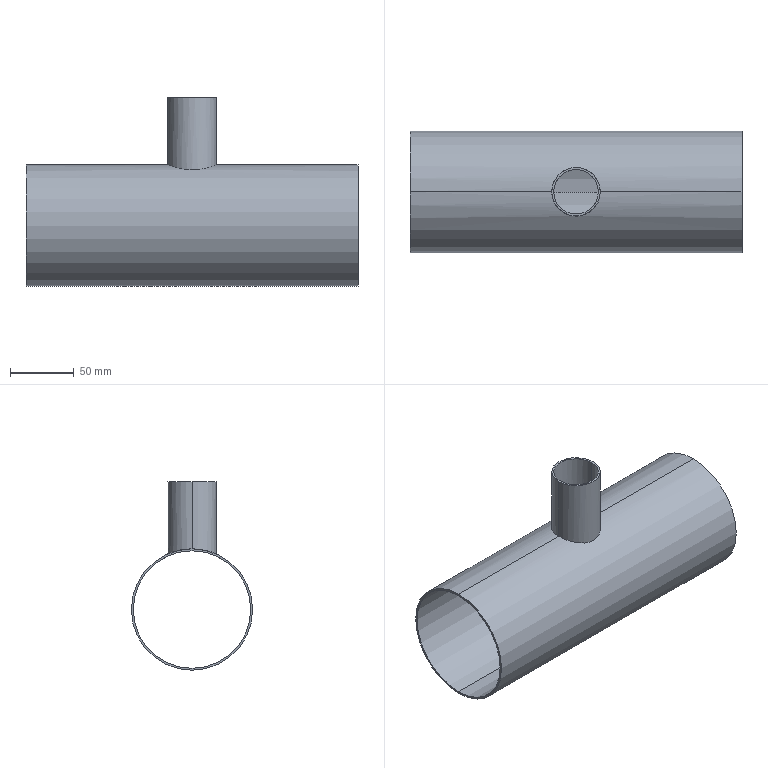Part | SolidWorks | features BaseBody 1 | 1 solid | 11 faces | box 260 x 95 x 147.5 mm | volume 122435 mm3 | cylinder 8 | plane 3 | commonest cylinder face diameters 35 x2 38 x2 92 x2 95 x2
STEP:
#1=CARTESIAN_POINT('',(-17.5,0.,46.));
#2=VERTEX_POINT('',#1);
#3=CARTESIAN_POINT('',(17.5,0.,46.));
#4=VERTEX_POINT('',#3);
#5=CARTESIAN_POINT('',(-17.5,0.,46.));
#6=CARTESIAN_POINT('',(-17.5,-1.168,46.));
#7=CARTESIAN_POINT('',(-17.384,-2.314,45.956));
#8=CARTESIAN_POINT('',(-17.046,-4.002,45.829));
#9=CARTESIAN_POINT('',(-16.905,-4.56,45.777));
#10=CARTESIAN_POINT('',(-16.568,-5.665,45.653));
#11=CARTESIAN_POINT('',(-16.371,-6.211,45.582));
#12=CARTESIAN_POINT('',(-15.709,-7.797,45.347));
#13=CARTESIAN_POINT('',(-15.171,-8.798,45.161));
#14=CARTESIAN_POINT('',(-14.218,-10.218,44.853));
#15=CARTESIAN_POINT('',(-13.875,-10.68,44.745));
#16=CARTESIAN_POINT('',(-13.152,-11.559,44.526));
#17=CARTESIAN_POINT('',(-12.771,-11.978,44.415));
#18=CARTESIAN_POINT('',(-11.572,-13.176,44.08));
#19=CARTESIAN_POINT('',(-10.697,-13.897,43.856));
#20=CARTESIAN_POINT('',(-8.793,-15.174,43.431));
#21=CARTESIAN_POINT('',(-7.793,-15.71,43.237));
#22=CARTESIAN_POINT('',(-6.218,-16.368,42.99));
#23=CARTESIAN_POINT('',(-5.681,-16.562,42.915));
#24=CARTESIAN_POINT('',(-4.581,-16.9,42.784));
#25=CARTESIAN_POINT('',(-4.015,-17.043,42.726));
#26=CARTESIAN_POINT('',(-2.318,-17.384,42.589));
#27=CARTESIAN_POINT('',(-1.175,-17.499,42.542));
#28=CARTESIAN_POINT('',(0.5549,-17.501,42.541));
#29=CARTESIAN_POINT('',(1.137,-17.473,42.552));
#30=CARTESIAN_POINT('',(2.295,-17.359,42.599));
#31=CARTESIAN_POINT('',(2.867,-17.273,42.634));
#32=CARTESIAN_POINT('',(4.557,-16.935,42.77));
#33=CARTESIAN_POINT('',(5.654,-16.602,42.902));
#34=CARTESIAN_POINT('',(7.786,-15.715,43.235));
#35=CARTESIAN_POINT('',(8.789,-15.175,43.43));
#36=CARTESIAN_POINT('',(10.203,-14.229,43.745));
#37=CARTESIAN_POINT('',(10.659,-13.891,43.854));
#38=CARTESIAN_POINT('',(11.541,-13.167,44.077));
#39=CARTESIAN_POINT('',(11.966,-12.783,44.19));
#40=CARTESIAN_POINT('',(13.169,-11.581,44.526));
#41=CARTESIAN_POINT('',(13.888,-10.709,44.747));
#42=CARTESIAN_POINT('',(14.84,-9.293,45.054));
#43=CARTESIAN_POINT('',(15.138,-8.799,45.153));
#44=CARTESIAN_POINT('',(15.681,-7.789,45.339));
#45=CARTESIAN_POINT('',(15.927,-7.274,45.424));
#46=CARTESIAN_POINT('',(16.586,-5.697,45.658));
#47=CARTESIAN_POINT('',(16.923,-4.604,45.783));
#48=CARTESIAN_POINT('',(17.268,-2.899,45.912));
#49=CARTESIAN_POINT('',(17.355,-2.321,45.945));
#50=CARTESIAN_POINT('',(17.471,-1.165,45.989));
#51=CARTESIAN_POINT('',(17.5,-0.584,46.));
#52=CARTESIAN_POINT('',(17.5,0.,46.));
#53=B_SPLINE_CURVE_WITH_KNOTS('',3,(#5,#6,#7,#8,#9,#10,#11,#12,#13,#14,#15,#16,#17,#18,#19,#20,#21,#22,#23,#24,#25,#26,#27,#28,#29,#30,#31,#32,#33,#34,#35,#36,#37,#38,#39,#40,#41,#42,#43,#44,#45,#46,#47,#48,#49,#50,#51,#52),.UNSPECIFIED.,.F.,.F.,(4,2,2,2,2,2,2,2,2,2,2,2,2,2,2,2,2,2,2,2,2,2,2,4),(0.,0.003451,0.005176,0.006902,0.01035,0.01208,0.0138,0.01725,0.02071,0.02243,0.02416,0.02761,0.02933,0.03106,0.03451,0.03796,0.03969,0.04141,0.04486,0.04659,0.04831,0.05176,0.05349,0.05521),.UNSPECIFIED.);
#54=EDGE_CURVE('',#2,#4,#53,.T.);
#55=ORIENTED_EDGE('',*,*,#54,.F.);
#56=CARTESIAN_POINT('',(-17.5,0.,100.));
#57=VERTEX_POINT('',#56);
#58=CARTESIAN_POINT('',(-17.5,0.,-47.501));
#59=DIRECTION('',(0.,0.,1.));
#60=VECTOR('',#59,1000.);
#61=LINE('',#58,#60);
#62=EDGE_CURVE('',#2,#57,#61,.T.);
#63=ORIENTED_EDGE('',*,*,#62,.T.);
#64=CARTESIAN_POINT('',(17.5,0.,100.));
#65=VERTEX_POINT('',#64);
#66=CARTESIAN_POINT('',(0.,0.,100.));
#67=DIRECTION('',(0.,0.,1.));
#68=DIRECTION('',(1.,0.,0.));
#69=AXIS2_PLACEMENT_3D('',#66,#67,#68);
#70=CIRCLE('',#69,17.5);
#71=EDGE_CURVE('',#57,#65,#70,.T.);
#72=ORIENTED_EDGE('',*,*,#71,.T.);
#73=CARTESIAN_POINT('',(17.5,0.,-47.501));
#74=DIRECTION('',(0.,0.,1.));
#75=VECTOR('',#74,1000.);
#76=LINE('',#73,#75);
#77=EDGE_CURVE('',#4,#65,#76,.T.);
#78=ORIENTED_EDGE('',*,*,#77,.F.);
#79=EDGE_LOOP('',(#55,#63,#72,#78));
#80=FACE_OUTER_BOUND('',#79,.T.);
#81=CARTESIAN_POINT('',(0.,0.,-47.501));
#82=DIRECTION('',(0.,0.,1.));
#83=DIRECTION('',(1.,0.,0.));
#84=AXIS2_PLACEMENT_3D('',#81,#82,#83);
#85=CYLINDRICAL_SURFACE('',#84,17.5);
#86=ADVANCED_FACE('',(#80),#85,.F.);
#87=CARTESIAN_POINT('',(19.,0.,47.5));
#88=VERTEX_POINT('',#87);
#89=CARTESIAN_POINT('',(-19.,0.,47.5));
#90=VERTEX_POINT('',#89);
#91=CARTESIAN_POINT('',(19.,0.,47.5));
#92=CARTESIAN_POINT('',(19.,1.269,47.5));
#93=CARTESIAN_POINT('',(18.874,2.515,47.449));
#94=CARTESIAN_POINT('',(18.506,4.349,47.304));
#95=CARTESIAN_POINT('',(18.353,4.955,47.245));
#96=CARTESIAN_POINT('',(18.078,5.856,47.139));
#97=CARTESIAN_POINT('',(17.978,6.155,47.1));
#98=CARTESIAN_POINT('',(17.765,6.744,47.02));
#99=CARTESIAN_POINT('',(17.652,7.035,46.977));
#100=CARTESIAN_POINT('',(17.053,8.47,46.753));
#101=CARTESIAN_POINT('',(16.468,9.556,46.541));
#102=CARTESIAN_POINT('',(15.435,11.098,46.188));
#103=CARTESIAN_POINT('',(15.062,11.598,46.065));
#104=CARTESIAN_POINT('',(14.277,12.551,45.814));
#105=CARTESIAN_POINT('',(13.864,13.006,45.687));
#106=CARTESIAN_POINT('',(12.998,13.872,45.431));
#107=CARTESIAN_POINT('',(12.544,14.284,45.303));
#108=CARTESIAN_POINT('',(11.595,15.064,45.05));
#109=CARTESIAN_POINT('',(11.098,15.434,44.924));
#110=CARTESIAN_POINT('',(9.55,16.472,44.558));
#111=CARTESIAN_POINT('',(8.465,17.055,44.336));
#112=CARTESIAN_POINT('',(6.756,17.769,44.052));
#113=CARTESIAN_POINT('',(6.173,17.98,43.966));
#114=CARTESIAN_POINT('',(4.978,18.347,43.814));
#115=CARTESIAN_POINT('',(4.363,18.503,43.748));
#116=CARTESIAN_POINT('',(2.52,18.874,43.59));
#117=CARTESIAN_POINT('',(1.279,18.998,43.535));
#118=CARTESIAN_POINT('',(-0.2884,19.,43.534));
#119=CARTESIAN_POINT('',(-0.6027,18.993,43.538));
#120=CARTESIAN_POINT('',(-1.233,18.963,43.551));
#121=CARTESIAN_POINT('',(-1.55,18.939,43.561));
#122=CARTESIAN_POINT('',(-2.494,18.846,43.601));
#123=CARTESIAN_POINT('',(-3.114,18.753,43.641));
#124=CARTESIAN_POINT('',(-4.951,18.386,43.798));
#125=CARTESIAN_POINT('',(-6.143,18.023,43.951));
#126=CARTESIAN_POINT('',(-8.458,17.06,44.334));
#127=CARTESIAN_POINT('',(-9.545,16.475,44.557));
#128=CARTESIAN_POINT('',(-11.079,15.448,44.919));
#129=CARTESIAN_POINT('',(-11.574,15.081,45.044));
#130=CARTESIAN_POINT('',(-12.532,14.295,45.3));
#131=CARTESIAN_POINT('',(-12.991,13.878,45.43));
#132=CARTESIAN_POINT('',(-14.296,12.576,45.814));
#133=CARTESIAN_POINT('',(-15.075,11.63,46.066));
#134=CARTESIAN_POINT('',(-16.11,10.092,46.418));
#135=CARTESIAN_POINT('',(-16.434,9.556,46.532));
#136=CARTESIAN_POINT('',(-17.023,8.462,46.744));
#137=CARTESIAN_POINT('',(-17.289,7.903,46.842));
#138=CARTESIAN_POINT('',(-18.005,6.191,47.109));
#139=CARTESIAN_POINT('',(-18.372,5.004,47.252));
#140=CARTESIAN_POINT('',(-18.748,3.149,47.4));
#141=CARTESIAN_POINT('',(-18.842,2.522,47.437));
#142=CARTESIAN_POINT('',(-18.968,1.266,47.487));
#143=CARTESIAN_POINT('',(-19.,0.6348,47.5));
#144=CARTESIAN_POINT('',(-19.,0.,47.5));
#145=B_SPLINE_CURVE_WITH_KNOTS('',3,(#91,#92,#93,#94,#95,#96,#97,#98,#99,#100,#101,#102,#103,#104,#105,#106,#107,#108,#109,#110,#111,#112,#113,#114,#115,#116,#117,#118,#119,#120,#121,#122,#123,#124,#125,#126,#127,#128,#129,#130,#131,#132,#133,#134,#135,#136,#137,#138,#139,#140,#141,#142,#143,#144),.UNSPECIFIED.,.F.,.F.,(4,2,2,2,2,2,2,2,2,2,2,2,2,2,2,2,2,2,2,2,2,2,2,2,2,2,4),(0.,0.003751,0.005626,0.006564,0.007501,0.01125,0.01313,0.015,0.01688,0.01875,0.0225,0.02438,0.02625,0.03001,0.03094,0.03188,0.03376,0.03751,0.04126,0.04313,0.04501,0.04876,0.05063,0.05251,0.05626,0.05814,0.06001),.UNSPECIFIED.);
#146=EDGE_CURVE('',#88,#90,#145,.T.);
#147=ORIENTED_EDGE('',*,*,#146,.T.);
#148=CARTESIAN_POINT('',(-19.,0.,100.));
#149=VERTEX_POINT('',#148);
#150=CARTESIAN_POINT('',(-19.,0.,-47.501));
#151=DIRECTION('',(0.,0.,1.));
#152=VECTOR('',#151,1000.);
#153=LINE('',#150,#152);
#154=EDGE_CURVE('',#90,#149,#153,.T.);
#155=ORIENTED_EDGE('',*,*,#154,.T.);
#156=CARTESIAN_POINT('',(19.,0.,100.));
#157=VERTEX_POINT('',#156);
#158=CARTESIAN_POINT('',(0.,0.,100.));
#159=DIRECTION('',(0.,0.,1.));
#160=DIRECTION('',(1.,0.,0.));
#161=AXIS2_PLACEMENT_3D('',#158,#159,#160);
#162=CIRCLE('',#161,19.);
#163=EDGE_CURVE('',#157,#149,#162,.T.);
#164=ORIENTED_EDGE('',*,*,#163,.F.);
#165=CARTESIAN_POINT('',(19.,0.,-47.501));
#166=DIRECTION('',(0.,0.,1.));
#167=VECTOR('',#166,1000.);
#168=LINE('',#165,#167);
#169=EDGE_CURVE('',#88,#157,#168,.T.);
#170=ORIENTED_EDGE('',*,*,#169,.F.);
#171=EDGE_LOOP('',(#147,#155,#164,#170));
#172=FACE_OUTER_BOUND('',#171,.T.);
#173=CARTESIAN_POINT('',(0.,0.,-47.501));
#174=DIRECTION('',(0.,0.,1.));
#175=DIRECTION('',(1.,0.,0.));
#176=AXIS2_PLACEMENT_3D('',#173,#174,#175);
#177=CYLINDRICAL_SURFACE('',#176,19.);
#178=ADVANCED_FACE('',(#172),#177,.T.);
#179=CARTESIAN_POINT('',(130.,0.,46.));
#180=VERTEX_POINT('',#179);
#181=CARTESIAN_POINT('',(130.,0.,-46.));
#182=VERTEX_POINT('',#181);
#183=CARTESIAN_POINT('',(130.,0.,0.));
#184=DIRECTION('',(1.,0.,0.));
#185=DIRECTION('',(0.,0.,-1.));
#186=AXIS2_PLACEMENT_3D('',#183,#184,#185);
#187=CIRCLE('',#186,46.);
#188=EDGE_CURVE('',#180,#182,#187,.T.);
#189=ORIENTED_EDGE('',*,*,#188,.T.);
#190=CARTESIAN_POINT('',(-130.,0.,-46.));
#191=VERTEX_POINT('',#190);
#192=CARTESIAN_POINT('',(130.,0.,-46.));
#193=DIRECTION('',(-1.,0.,0.));
#194=VECTOR('',#193,1000.);
#195=LINE('',#192,#194);
#196=EDGE_CURVE('',#182,#191,#195,.T.);
#197=ORIENTED_EDGE('',*,*,#196,.T.);
#198=CARTESIAN_POINT('',(-130.,0.,46.));
#199=VERTEX_POINT('',#198);
#200=CARTESIAN_POINT('',(-130.,0.,0.));
#201=DIRECTION('',(1.,0.,0.));
#202=DIRECTION('',(0.,0.,-1.));
#203=AXIS2_PLACEMENT_3D('',#200,#201,#202);
#204=CIRCLE('',#203,46.);
#205=EDGE_CURVE('',#199,#191,#204,.T.);
#206=ORIENTED_EDGE('',*,*,#205,.F.);
#207=CARTESIAN_POINT('',(130.,0.,46.));
#208=DIRECTION('',(-1.,0.,0.));
#209=VECTOR('',#208,1000.);
#210=LINE('',#207,#209);
#211=EDGE_CURVE('',#2,#199,#210,.T.);
#212=ORIENTED_EDGE('',*,*,#211,.F.);
#213=ORIENTED_EDGE('',*,*,#54,.T.);
#214=CARTESIAN_POINT('',(130.,0.,46.));
#215=DIRECTION('',(-1.,0.,0.));
#216=VECTOR('',#215,1000.);
#217=LINE('',#214,#216);
#218=EDGE_CURVE('',#180,#4,#217,.T.);
#219=ORIENTED_EDGE('',*,*,#218,.F.);
#220=EDGE_LOOP('',(#189,#197,#206,#212,#213,#219));
#221=FACE_OUTER_BOUND('',#220,.T.);
#222=CARTESIAN_POINT('',(130.,0.,0.));
#223=DIRECTION('',(-1.,0.,0.));
#224=DIRECTION('',(0.,0.,1.));
#225=AXIS2_PLACEMENT_3D('',#222,#223,#224);
#226=CYLINDRICAL_SURFACE('',#225,46.);
#227=ADVANCED_FACE('',(#221),#226,.F.);
#228=CARTESIAN_POINT('',(130.,0.,-47.5));
#229=VERTEX_POINT('',#228);
#230=CARTESIAN_POINT('',(130.,0.,47.5));
#231=VERTEX_POINT('',#230);
#232=CARTESIAN_POINT('',(130.,0.,0.));
#233=DIRECTION('',(1.,0.,0.));
#234=DIRECTION('',(0.,0.,-1.));
#235=AXIS2_PLACEMENT_3D('',#232,#233,#234);
#236=CIRCLE('',#235,47.5);
#237=EDGE_CURVE('',#229,#231,#236,.T.);
#238=ORIENTED_EDGE('',*,*,#237,.F.);
#239=CARTESIAN_POINT('',(-130.,0.,-47.5));
#240=VERTEX_POINT('',#239);
#241=CARTESIAN_POINT('',(130.,0.,-47.5));
#242=DIRECTION('',(-1.,0.,0.));
#243=VECTOR('',#242,1000.);
#244=LINE('',#241,#243);
#245=EDGE_CURVE('',#229,#240,#244,.T.);
#246=ORIENTED_EDGE('',*,*,#245,.T.);
#247=CARTESIAN_POINT('',(-130.,0.,47.5));
#248=VERTEX_POINT('',#247);
#249=CARTESIAN_POINT('',(-130.,0.,0.));
#250=DIRECTION('',(1.,0.,0.));
#251=DIRECTION('',(0.,0.,-1.));
#252=AXIS2_PLACEMENT_3D('',#249,#250,#251);
#253=CIRCLE('',#252,47.5);
#254=EDGE_CURVE('',#240,#248,#253,.T.);
#255=ORIENTED_EDGE('',*,*,#254,.T.);
#256=CARTESIAN_POINT('',(130.,0.,47.5));
#257=DIRECTION('',(-1.,0.,0.));
#258=VECTOR('',#257,1000.);
#259=LINE('',#256,#258);
#260=EDGE_CURVE('',#90,#248,#259,.T.);
#261=ORIENTED_EDGE('',*,*,#260,.F.);
#262=ORIENTED_EDGE('',*,*,#146,.F.);
#263=CARTESIAN_POINT('',(130.,0.,47.5));
#264=DIRECTION('',(-1.,0.,0.));
#265=VECTOR('',#264,1000.);
#266=LINE('',#263,#265);
#267=EDGE_CURVE('',#231,#88,#266,.T.);
#268=ORIENTED_EDGE('',*,*,#267,.F.);
#269=EDGE_LOOP('',(#238,#246,#255,#261,#262,#268));
#270=FACE_OUTER_BOUND('',#269,.T.);
#271=CARTESIAN_POINT('',(130.,0.,0.));
#272=DIRECTION('',(-1.,0.,0.));
#273=DIRECTION('',(0.,0.,1.));
#274=AXIS2_PLACEMENT_3D('',#271,#272,#273);
#275=CYLINDRICAL_SURFACE('',#274,47.5);
#276=ADVANCED_FACE('',(#270),#275,.T.);
#277=CARTESIAN_POINT('',(0.,0.,100.));
#278=DIRECTION('',(0.,0.,1.));
#279=DIRECTION('',(1.,0.,0.));
#280=AXIS2_PLACEMENT_3D('',#277,#278,#279);
#281=CIRCLE('',#280,17.5);
#282=EDGE_CURVE('',#65,#57,#281,.T.);
#283=ORIENTED_EDGE('',*,*,#282,.F.);
#284=ORIENTED_EDGE('',*,*,#71,.F.);
#285=EDGE_LOOP('',(#283,#284));
#286=FACE_BOUND('',#285,.T.);
#287=ORIENTED_EDGE('',*,*,#163,.T.);
#288=CARTESIAN_POINT('',(0.,0.,100.));
#289=DIRECTION('',(0.,0.,1.));
#290=DIRECTION('',(1.,0.,0.));
#291=AXIS2_PLACEMENT_3D('',#288,#289,#290);
#292=CIRCLE('',#291,19.);
#293=EDGE_CURVE('',#149,#157,#292,.T.);
#294=ORIENTED_EDGE('',*,*,#293,.T.);
#295=EDGE_LOOP('',(#287,#294));
#296=FACE_OUTER_BOUND('',#295,.T.);
#297=CARTESIAN_POINT('',(0.,0.,100.));
#298=DIRECTION('',(0.,0.,1.));
#299=DIRECTION('',(1.,0.,0.));
#300=AXIS2_PLACEMENT_3D('',#297,#298,#299);
#301=PLANE('',#300);
#302=ADVANCED_FACE('',(#286,#296),#301,.T.);
#303=ORIENTED_EDGE('',*,*,#205,.T.);
#304=CARTESIAN_POINT('',(-130.,0.,0.));
#305=DIRECTION('',(1.,0.,0.));
#306=DIRECTION('',(0.,0.,-1.));
#307=AXIS2_PLACEMENT_3D('',#304,#305,#306);
#308=CIRCLE('',#307,46.);
#309=EDGE_CURVE('',#191,#199,#308,.T.);
#310=ORIENTED_EDGE('',*,*,#309,.T.);
#311=EDGE_LOOP('',(#303,#310));
#312=FACE_BOUND('',#311,.T.);
#313=CARTESIAN_POINT('',(-130.,0.,0.));
#314=DIRECTION('',(1.,0.,0.));
#315=DIRECTION('',(0.,0.,-1.));
#316=AXIS2_PLACEMENT_3D('',#313,#314,#315);
#317=CIRCLE('',#316,47.5);
#318=EDGE_CURVE('',#248,#240,#317,.T.);
#319=ORIENTED_EDGE('',*,*,#318,.F.);
#320=ORIENTED_EDGE('',*,*,#254,.F.);
#321=EDGE_LOOP('',(#319,#320));
#322=FACE_OUTER_BOUND('',#321,.T.);
#323=CARTESIAN_POINT('',(-130.,0.,0.));
#324=DIRECTION('',(1.,0.,0.));
#325=DIRECTION('',(0.,1.,0.));
#326=AXIS2_PLACEMENT_3D('',#323,#324,#325);
#327=PLANE('',#326);
#328=ADVANCED_FACE('',(#312,#322),#327,.F.);
#329=ORIENTED_EDGE('',*,*,#188,.F.);
#330=CARTESIAN_POINT('',(130.,0.,0.));
#331=DIRECTION('',(1.,0.,0.));
#332=DIRECTION('',(0.,0.,-1.));
#333=AXIS2_PLACEMENT_3D('',#330,#331,#332);
#334=CIRCLE('',#333,46.);
#335=EDGE_CURVE('',#182,#180,#334,.T.);
#336=ORIENTED_EDGE('',*,*,#335,.F.);
#337=EDGE_LOOP('',(#329,#336));
#338=FACE_BOUND('',#337,.T.);
#339=CARTESIAN_POINT('',(130.,0.,0.));
#340=DIRECTION('',(1.,0.,0.));
#341=DIRECTION('',(0.,0.,-1.));
#342=AXIS2_PLACEMENT_3D('',#339,#340,#341);
#343=CIRCLE('',#342,47.5);
#344=EDGE_CURVE('',#231,#229,#343,.T.);
#345=ORIENTED_EDGE('',*,*,#344,.T.);
#346=ORIENTED_EDGE('',*,*,#237,.T.);
#347=EDGE_LOOP('',(#345,#346));
#348=FACE_OUTER_BOUND('',#347,.T.);
#349=CARTESIAN_POINT('',(130.,0.,0.));
#350=DIRECTION('',(1.,0.,0.));
#351=DIRECTION('',(0.,1.,0.));
#352=AXIS2_PLACEMENT_3D('',#349,#350,#351);
#353=PLANE('',#352);
#354=ADVANCED_FACE('',(#338,#348),#353,.T.);
#355=ORIENTED_EDGE('',*,*,#245,.F.);
#356=ORIENTED_EDGE('',*,*,#344,.F.);
#357=ORIENTED_EDGE('',*,*,#267,.T.);
#358=CARTESIAN_POINT('',(-19.,0.,47.5));
#359=CARTESIAN_POINT('',(-19.,-1.269,47.5));
#360=CARTESIAN_POINT('',(-18.874,-2.515,47.449));
#361=CARTESIAN_POINT('',(-18.506,-4.349,47.304));
#362=CARTESIAN_POINT('',(-18.353,-4.955,47.245));
#363=CARTESIAN_POINT('',(-18.078,-5.856,47.139));
#364=CARTESIAN_POINT('',(-17.978,-6.155,47.1));
#365=CARTESIAN_POINT('',(-17.765,-6.744,47.02));
#366=CARTESIAN_POINT('',(-17.652,-7.035,46.977));
#367=CARTESIAN_POINT('',(-17.053,-8.47,46.753));
#368=CARTESIAN_POINT('',(-16.468,-9.556,46.541));
#369=CARTESIAN_POINT('',(-15.435,-11.098,46.188));
#370=CARTESIAN_POINT('',(-15.062,-11.598,46.065));
#371=CARTESIAN_POINT('',(-14.277,-12.551,45.814));
#372=CARTESIAN_POINT('',(-13.864,-13.006,45.687));
#373=CARTESIAN_POINT('',(-12.998,-13.872,45.431));
#374=CARTESIAN_POINT('',(-12.544,-14.284,45.303));
#375=CARTESIAN_POINT('',(-11.595,-15.064,45.05));
#376=CARTESIAN_POINT('',(-11.098,-15.434,44.924));
#377=CARTESIAN_POINT('',(-9.55,-16.472,44.558));
#378=CARTESIAN_POINT('',(-8.465,-17.055,44.336));
#379=CARTESIAN_POINT('',(-6.756,-17.769,44.052));
#380=CARTESIAN_POINT('',(-6.173,-17.98,43.966));
#381=CARTESIAN_POINT('',(-4.978,-18.347,43.814));
#382=CARTESIAN_POINT('',(-4.363,-18.503,43.748));
#383=CARTESIAN_POINT('',(-2.52,-18.874,43.59));
#384=CARTESIAN_POINT('',(-1.279,-18.998,43.535));
#385=CARTESIAN_POINT('',(0.2884,-19.,43.534));
#386=CARTESIAN_POINT('',(0.6027,-18.993,43.538));
#387=CARTESIAN_POINT('',(1.233,-18.963,43.551));
#388=CARTESIAN_POINT('',(1.55,-18.939,43.561));
#389=CARTESIAN_POINT('',(2.494,-18.846,43.601));
#390=CARTESIAN_POINT('',(3.114,-18.753,43.641));
#391=CARTESIAN_POINT('',(4.951,-18.386,43.798));
#392=CARTESIAN_POINT('',(6.143,-18.023,43.951));
#393=CARTESIAN_POINT('',(8.458,-17.06,44.334));
#394=CARTESIAN_POINT('',(9.545,-16.475,44.557));
#395=CARTESIAN_POINT('',(11.079,-15.448,44.919));
#396=CARTESIAN_POINT('',(11.574,-15.081,45.044));
#397=CARTESIAN_POINT('',(12.532,-14.295,45.3));
#398=CARTESIAN_POINT('',(12.991,-13.878,45.43));
#399=CARTESIAN_POINT('',(14.296,-12.576,45.814));
#400=CARTESIAN_POINT('',(15.075,-11.63,46.066));
#401=CARTESIAN_POINT('',(16.11,-10.092,46.418));
#402=CARTESIAN_POINT('',(16.434,-9.556,46.532));
#403=CARTESIAN_POINT('',(17.023,-8.462,46.744));
#404=CARTESIAN_POINT('',(17.289,-7.903,46.842));
#405=CARTESIAN_POINT('',(18.005,-6.191,47.109));
#406=CARTESIAN_POINT('',(18.372,-5.004,47.252));
#407=CARTESIAN_POINT('',(18.748,-3.149,47.4));
#408=CARTESIAN_POINT('',(18.842,-2.522,47.437));
#409=CARTESIAN_POINT('',(18.968,-1.266,47.487));
#410=CARTESIAN_POINT('',(19.,-0.6344,47.5));
#411=CARTESIAN_POINT('',(19.,0.,47.5));
#412=B_SPLINE_CURVE_WITH_KNOTS('',3,(#358,#359,#360,#361,#362,#363,#364,#365,#366,#367,#368,#369,#370,#371,#372,#373,#374,#375,#376,#377,#378,#379,#380,#381,#382,#383,#384,#385,#386,#387,#388,#389,#390,#391,#392,#393,#394,#395,#396,#397,#398,#399,#400,#401,#402,#403,#404,#405,#406,#407,#408,#409,#410,#411),.UNSPECIFIED.,.F.,.F.,(4,2,2,2,2,2,2,2,2,2,2,2,2,2,2,2,2,2,2,2,2,2,2,2,2,2,4),(0.06001,0.06376,0.06564,0.06657,0.06751,0.07126,0.07313,0.07501,0.07688,0.07876,0.08251,0.08438,0.08626,0.09001,0.09095,0.09188,0.09376,0.09751,0.1013,0.1031,0.105,0.1088,0.1106,0.1125,0.1163,0.1181,0.12),.UNSPECIFIED.);
#413=EDGE_CURVE('',#90,#88,#412,.T.);
#414=ORIENTED_EDGE('',*,*,#413,.F.);
#415=ORIENTED_EDGE('',*,*,#260,.T.);
#416=ORIENTED_EDGE('',*,*,#318,.T.);
#417=EDGE_LOOP('',(#355,#356,#357,#414,#415,#416));
#418=FACE_OUTER_BOUND('',#417,.T.);
#419=CARTESIAN_POINT('',(130.,0.,0.));
#420=DIRECTION('',(-1.,0.,0.));
#421=DIRECTION('',(0.,0.,1.));
#422=AXIS2_PLACEMENT_3D('',#419,#420,#421);
#423=CYLINDRICAL_SURFACE('',#422,47.5);
#424=ADVANCED_FACE('',(#418),#423,.T.);
#425=ORIENTED_EDGE('',*,*,#196,.F.);
#426=ORIENTED_EDGE('',*,*,#335,.T.);
#427=ORIENTED_EDGE('',*,*,#218,.T.);
#428=CARTESIAN_POINT('',(17.5,0.,46.));
#429=CARTESIAN_POINT('',(17.5,1.168,46.));
#430=CARTESIAN_POINT('',(17.384,2.314,45.956));
#431=CARTESIAN_POINT('',(17.046,4.002,45.829));
#432=CARTESIAN_POINT('',(16.905,4.56,45.777));
#433=CARTESIAN_POINT('',(16.568,5.665,45.653));
#434=CARTESIAN_POINT('',(16.371,6.211,45.582));
#435=CARTESIAN_POINT('',(15.709,7.797,45.347));
#436=CARTESIAN_POINT('',(15.171,8.798,45.161));
#437=CARTESIAN_POINT('',(14.218,10.218,44.853));
#438=CARTESIAN_POINT('',(13.875,10.68,44.745));
#439=CARTESIAN_POINT('',(13.152,11.559,44.526));
#440=CARTESIAN_POINT('',(12.771,11.978,44.415));
#441=CARTESIAN_POINT('',(11.572,13.176,44.08));
#442=CARTESIAN_POINT('',(10.697,13.897,43.856));
#443=CARTESIAN_POINT('',(8.793,15.174,43.431));
#444=CARTESIAN_POINT('',(7.793,15.71,43.237));
#445=CARTESIAN_POINT('',(6.218,16.368,42.99));
#446=CARTESIAN_POINT('',(5.681,16.562,42.915));
#447=CARTESIAN_POINT('',(4.581,16.9,42.784));
#448=CARTESIAN_POINT('',(4.015,17.043,42.726));
#449=CARTESIAN_POINT('',(2.318,17.384,42.589));
#450=CARTESIAN_POINT('',(1.175,17.499,42.542));
#451=CARTESIAN_POINT('',(-0.5549,17.501,42.541));
#452=CARTESIAN_POINT('',(-1.137,17.473,42.552));
#453=CARTESIAN_POINT('',(-2.295,17.359,42.599));
#454=CARTESIAN_POINT('',(-2.867,17.273,42.634));
#455=CARTESIAN_POINT('',(-4.557,16.935,42.77));
#456=CARTESIAN_POINT('',(-5.654,16.602,42.902));
#457=CARTESIAN_POINT('',(-7.786,15.715,43.235));
#458=CARTESIAN_POINT('',(-8.789,15.175,43.43));
#459=CARTESIAN_POINT('',(-10.203,14.229,43.745));
#460=CARTESIAN_POINT('',(-10.659,13.891,43.854));
#461=CARTESIAN_POINT('',(-11.541,13.167,44.077));
#462=CARTESIAN_POINT('',(-11.966,12.783,44.19));
#463=CARTESIAN_POINT('',(-13.169,11.581,44.526));
#464=CARTESIAN_POINT('',(-13.888,10.709,44.747));
#465=CARTESIAN_POINT('',(-14.84,9.293,45.054));
#466=CARTESIAN_POINT('',(-15.138,8.799,45.153));
#467=CARTESIAN_POINT('',(-15.681,7.789,45.339));
#468=CARTESIAN_POINT('',(-15.927,7.274,45.424));
#469=CARTESIAN_POINT('',(-16.586,5.697,45.658));
#470=CARTESIAN_POINT('',(-16.923,4.604,45.783));
#471=CARTESIAN_POINT('',(-17.268,2.899,45.912));
#472=CARTESIAN_POINT('',(-17.355,2.321,45.945));
#473=CARTESIAN_POINT('',(-17.471,1.165,45.989));
#474=CARTESIAN_POINT('',(-17.5,0.5837,46.));
#475=CARTESIAN_POINT('',(-17.5,0.,46.));
#476=B_SPLINE_CURVE_WITH_KNOTS('',3,(#428,#429,#430,#431,#432,#433,#434,#435,#436,#437,#438,#439,#440,#441,#442,#443,#444,#445,#446,#447,#448,#449,#450,#451,#452,#453,#454,#455,#456,#457,#458,#459,#460,#461,#462,#463,#464,#465,#466,#467,#468,#469,#470,#471,#472,#473,#474,#475),.UNSPECIFIED.,.F.,.F.,(4,2,2,2,2,2,2,2,2,2,2,2,2,2,2,2,2,2,2,2,2,2,2,4),(0.05521,0.05867,0.06039,0.06212,0.06557,0.06729,0.06902,0.07247,0.07592,0.07764,0.07937,0.08282,0.08454,0.08627,0.08972,0.09317,0.09489,0.09662,0.1001,0.1018,0.1035,0.107,0.1087,0.1104),.UNSPECIFIED.);
#477=EDGE_CURVE('',#4,#2,#476,.T.);
#478=ORIENTED_EDGE('',*,*,#477,.T.);
#479=ORIENTED_EDGE('',*,*,#211,.T.);
#480=ORIENTED_EDGE('',*,*,#309,.F.);
#481=EDGE_LOOP('',(#425,#426,#427,#478,#479,#480));
#482=FACE_OUTER_BOUND('',#481,.T.);
#483=CARTESIAN_POINT('',(130.,0.,0.));
#484=DIRECTION('',(-1.,0.,0.));
#485=DIRECTION('',(0.,0.,1.));
#486=AXIS2_PLACEMENT_3D('',#483,#484,#485);
#487=CYLINDRICAL_SURFACE('',#486,46.);
#488=ADVANCED_FACE('',(#482),#487,.F.);
#489=ORIENTED_EDGE('',*,*,#154,.F.);
#490=ORIENTED_EDGE('',*,*,#413,.T.);
#491=ORIENTED_EDGE('',*,*,#169,.T.);
#492=ORIENTED_EDGE('',*,*,#293,.F.);
#493=EDGE_LOOP('',(#489,#490,#491,#492));
#494=FACE_OUTER_BOUND('',#493,.T.);
#495=CARTESIAN_POINT('',(0.,0.,-47.501));
#496=DIRECTION('',(0.,0.,1.));
#497=DIRECTION('',(1.,0.,0.));
#498=AXIS2_PLACEMENT_3D('',#495,#496,#497);
#499=CYLINDRICAL_SURFACE('',#498,19.);
#500=ADVANCED_FACE('',(#494),#499,.T.);
#501=ORIENTED_EDGE('',*,*,#62,.F.);
#502=ORIENTED_EDGE('',*,*,#477,.F.);
#503=ORIENTED_EDGE('',*,*,#77,.T.);
#504=ORIENTED_EDGE('',*,*,#282,.T.);
#505=EDGE_LOOP('',(#501,#502,#503,#504));
#506=FACE_OUTER_BOUND('',#505,.T.);
#507=CARTESIAN_POINT('',(0.,0.,-47.501));
#508=DIRECTION('',(0.,0.,1.));
#509=DIRECTION('',(1.,0.,0.));
#510=AXIS2_PLACEMENT_3D('',#507,#508,#509);
#511=CYLINDRICAL_SURFACE('',#510,17.5);
#512=ADVANCED_FACE('',(#506),#511,.F.);
#513=CLOSED_SHELL('',(#86,#178,#227,#276,#302,#328,#354,#424,#488,#500,#512));
#514=MANIFOLD_SOLID_BREP('',#513);
#515=CARTESIAN_POINT('',(0.,0.,0.));
#516=DIRECTION('',(0.,0.,1.));
#517=DIRECTION('',(1.,0.,0.));
#518=AXIS2_PLACEMENT_3D('',#515,#516,#517);
#519=(LENGTH_UNIT()NAMED_UNIT(*)SI_UNIT(.MILLI.,.METRE.));
#520=UNCERTAINTY_MEASURE_WITH_UNIT(LENGTH_MEASURE(0.00001),#519,'','');
#521=(NAMED_UNIT(*)PLANE_ANGLE_UNIT()SI_UNIT($,.RADIAN.));
#522=(NAMED_UNIT(*)SI_UNIT($,.STERADIAN.)SOLID_ANGLE_UNIT());
#523=(GEOMETRIC_REPRESENTATION_CONTEXT(3)GLOBAL_UNCERTAINTY_ASSIGNED_CONTEXT((#520))GLOBAL_UNIT_ASSIGNED_CONTEXT((#519,#521,#522))REPRESENTATION_CONTEXT('',''));
#524=ADVANCED_BREP_SHAPE_REPRESENTATION('',(#514,#518),#523);